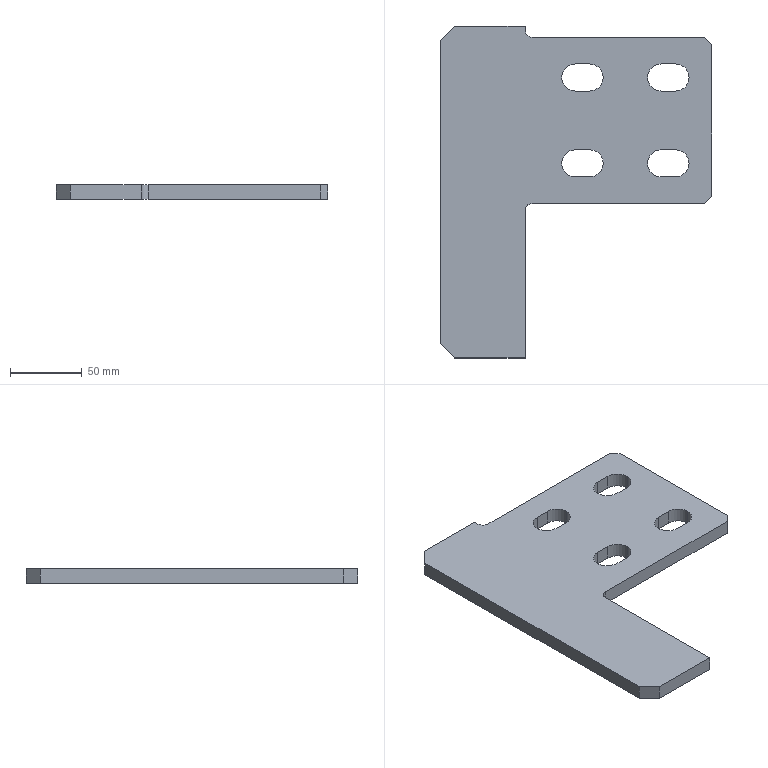Part | STEP file | 筋Plate-250×125-150 | 1 solid | 36 faces | box 190 x 232 x 10 mm | volume 269336 mm3 | plane 22 | cylinder 14 | commonest cylinder face diameters 19 x12 10 x2